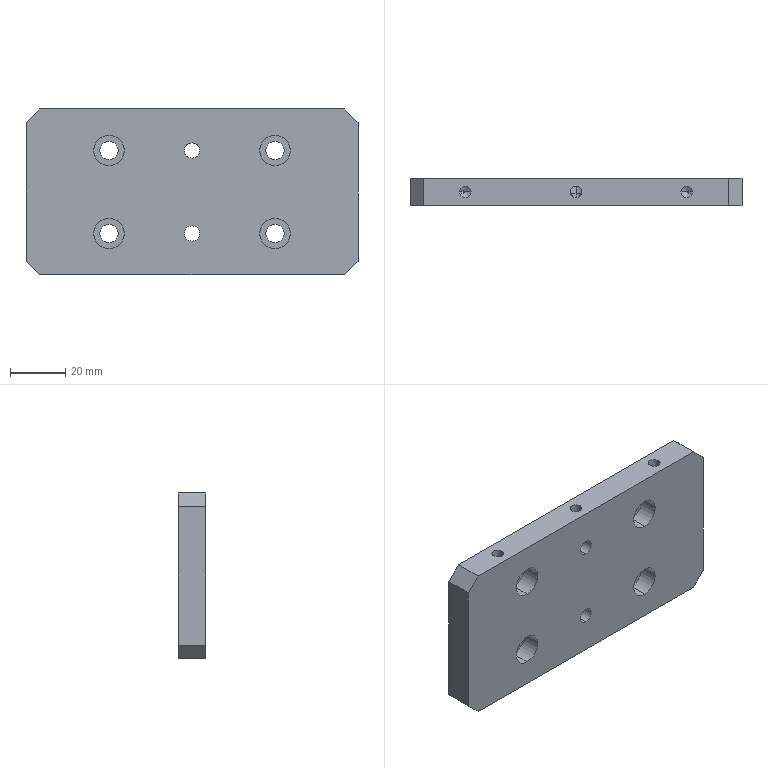Part | SolidWorks | features HoleWzd 3, Chamfer 1, Extrusion 1 | 1 solid | 52 faces | box 120 x 10 x 60 mm | volume 66873 mm3 | cylinder 30 | plane 16 | cone 6 | commonest cylinder face diameters 6.6 x8 11 x8 4.2 x6 5.5 x4 10 x4